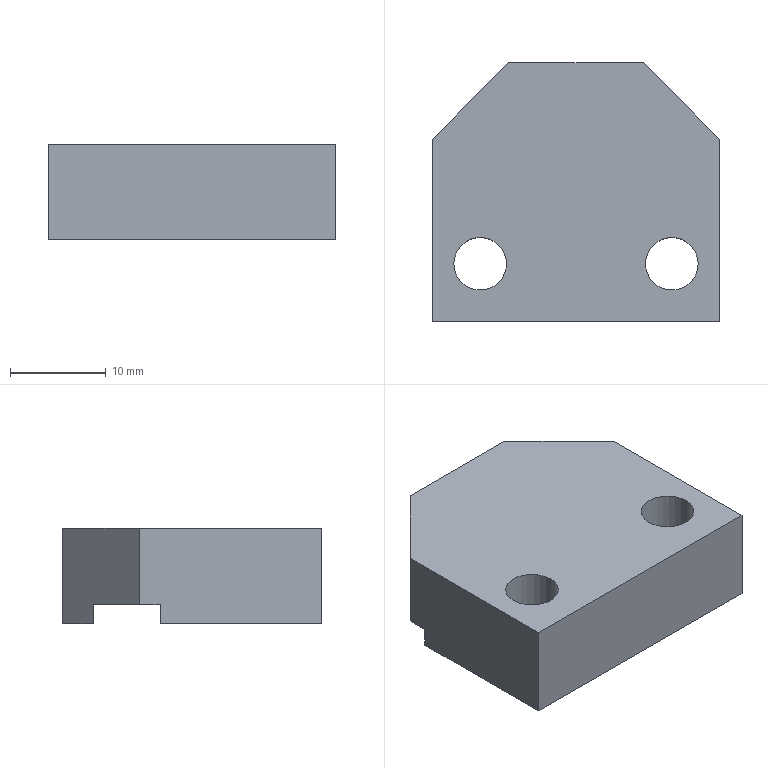Part | STEP file | detection track cover plate | 1 solid | 16 faces | box 30 x 27 x 10 mm | volume 6611 mm3 | plane 12 | cylinder 4 | commonest cylinder face diameters 5.5 x4
STEP:
#1=CARTESIAN_POINT('',(0.,0.,0.));
#2=DIRECTION('',(0.,0.,1.));
#3=DIRECTION('',(1.,0.,0.));
#4=AXIS2_PLACEMENT_3D('',#1,#2,#3);
#5=CARTESIAN_POINT('',(-12.75,-7.5,10.));
#6=VERTEX_POINT('',#5);
#7=CARTESIAN_POINT('',(-12.75,-7.5,0.));
#8=VERTEX_POINT('',#7);
#9=CARTESIAN_POINT('',(-12.75,-7.5,10.));
#10=DIRECTION('',(0.,0.,-1.));
#11=VECTOR('',#10,1.);
#12=LINE('',#9,#11);
#13=CARTESIAN_POINT('',(-10.,-7.5,10.));
#14=DIRECTION('',(0.,0.,-1.));
#15=DIRECTION('',(-1.,0.,0.));
#16=AXIS2_PLACEMENT_3D('',#13,#14,#15);
#17=CYLINDRICAL_SURFACE('',#16,2.75);
#18=CARTESIAN_POINT('',(6.283,0.));
#19=DIRECTION('',(0.,1.));
#20=VECTOR('',#19,1.);
#21=LINE('',#18,#20);
#22=(GEOMETRIC_REPRESENTATION_CONTEXT(2)PARAMETRIC_REPRESENTATION_CONTEXT()REPRESENTATION_CONTEXT('',''));
#23=DEFINITIONAL_REPRESENTATION('',(#21),#22);
#24=PCURVE('',#17,#23);
#25=CARTESIAN_POINT('',(-10.,-7.5,10.));
#26=DIRECTION('',(0.,0.,-1.));
#27=DIRECTION('',(-1.,0.,0.));
#28=AXIS2_PLACEMENT_3D('',#25,#26,#27);
#29=CYLINDRICAL_SURFACE('',#28,2.75);
#30=CARTESIAN_POINT('',(0.,0.));
#31=DIRECTION('',(0.,1.));
#32=VECTOR('',#31,1.);
#33=LINE('',#30,#32);
#34=(GEOMETRIC_REPRESENTATION_CONTEXT(2)PARAMETRIC_REPRESENTATION_CONTEXT()REPRESENTATION_CONTEXT('',''));
#35=DEFINITIONAL_REPRESENTATION('',(#33),#34);
#36=PCURVE('',#29,#35);
#37=SURFACE_CURVE('',#12,(#24,#36),.PCURVE_S1.);
#38=EDGE_CURVE('',#6,#8,#37,.T.);
#39=ORIENTED_EDGE('',*,*,#38,.T.);
#40=CARTESIAN_POINT('',(-7.25,-7.5,0.));
#41=VERTEX_POINT('',#40);
#42=CARTESIAN_POINT('',(-10.,-7.5,0.));
#43=DIRECTION('',(0.,0.,1.));
#44=DIRECTION('',(1.,0.,0.));
#45=AXIS2_PLACEMENT_3D('',#42,#43,#44);
#46=CIRCLE('',#45,2.75);
#47=CARTESIAN_POINT('',(9.425,10.));
#48=DIRECTION('',(-1.,0.));
#49=VECTOR('',#48,1.);
#50=LINE('',#47,#49);
#51=(GEOMETRIC_REPRESENTATION_CONTEXT(2)PARAMETRIC_REPRESENTATION_CONTEXT()REPRESENTATION_CONTEXT('',''));
#52=DEFINITIONAL_REPRESENTATION('',(#50),#51);
#53=PCURVE('',#17,#52);
#54=CARTESIAN_POINT('',(15.,-13.5,0.));
#55=DIRECTION('',(0.,0.,1.));
#56=DIRECTION('',(1.,0.,0.));
#57=AXIS2_PLACEMENT_3D('',#54,#55,#56);
#58=PLANE('',#57);
#59=CARTESIAN_POINT('',(-25.,6.));
#60=DIRECTION('',(1.,0.));
#61=AXIS2_PLACEMENT_2D('',#59,#60);
#62=CIRCLE('',#61,2.75);
#63=(GEOMETRIC_REPRESENTATION_CONTEXT(2)PARAMETRIC_REPRESENTATION_CONTEXT()REPRESENTATION_CONTEXT('',''));
#64=DEFINITIONAL_REPRESENTATION('',(#62),#63);
#65=PCURVE('',#58,#64);
#66=SURFACE_CURVE('',#46,(#53,#65),.PCURVE_S1.);
#67=EDGE_CURVE('',#8,#41,#66,.T.);
#68=ORIENTED_EDGE('',*,*,#67,.T.);
#69=CARTESIAN_POINT('',(-7.25,-7.5,10.));
#70=VERTEX_POINT('',#69);
#71=CARTESIAN_POINT('',(-7.25,-7.5,10.));
#72=DIRECTION('',(0.,0.,-1.));
#73=VECTOR('',#72,1.);
#74=LINE('',#71,#73);
#75=CARTESIAN_POINT('',(3.142,0.));
#76=DIRECTION('',(0.,1.));
#77=VECTOR('',#76,1.);
#78=LINE('',#75,#77);
#79=(GEOMETRIC_REPRESENTATION_CONTEXT(2)PARAMETRIC_REPRESENTATION_CONTEXT()REPRESENTATION_CONTEXT('',''));
#80=DEFINITIONAL_REPRESENTATION('',(#78),#79);
#81=PCURVE('',#17,#80);
#82=CARTESIAN_POINT('',(3.142,0.));
#83=DIRECTION('',(0.,1.));
#84=VECTOR('',#83,1.);
#85=LINE('',#82,#84);
#86=(GEOMETRIC_REPRESENTATION_CONTEXT(2)PARAMETRIC_REPRESENTATION_CONTEXT()REPRESENTATION_CONTEXT('',''));
#87=DEFINITIONAL_REPRESENTATION('',(#85),#86);
#88=PCURVE('',#29,#87);
#89=SURFACE_CURVE('',#74,(#81,#88),.PCURVE_S1.);
#90=EDGE_CURVE('',#70,#41,#89,.T.);
#91=ORIENTED_EDGE('',*,*,#90,.F.);
#92=CARTESIAN_POINT('',(-10.,-7.5,10.));
#93=DIRECTION('',(0.,0.,1.));
#94=DIRECTION('',(1.,0.,0.));
#95=AXIS2_PLACEMENT_3D('',#92,#93,#94);
#96=CIRCLE('',#95,2.75);
#97=CARTESIAN_POINT('',(9.425,0.));
#98=DIRECTION('',(-1.,0.));
#99=VECTOR('',#98,1.);
#100=LINE('',#97,#99);
#101=(GEOMETRIC_REPRESENTATION_CONTEXT(2)PARAMETRIC_REPRESENTATION_CONTEXT()REPRESENTATION_CONTEXT('',''));
#102=DEFINITIONAL_REPRESENTATION('',(#100),#101);
#103=PCURVE('',#17,#102);
#104=CARTESIAN_POINT('',(15.,-13.5,10.));
#105=DIRECTION('',(0.,0.,1.));
#106=DIRECTION('',(1.,0.,0.));
#107=AXIS2_PLACEMENT_3D('',#104,#105,#106);
#108=PLANE('',#107);
#109=CARTESIAN_POINT('',(-25.,6.));
#110=DIRECTION('',(1.,0.));
#111=AXIS2_PLACEMENT_2D('',#109,#110);
#112=CIRCLE('',#111,2.75);
#113=(GEOMETRIC_REPRESENTATION_CONTEXT(2)PARAMETRIC_REPRESENTATION_CONTEXT()REPRESENTATION_CONTEXT('',''));
#114=DEFINITIONAL_REPRESENTATION('',(#112),#113);
#115=PCURVE('',#108,#114);
#116=SURFACE_CURVE('',#96,(#103,#115),.PCURVE_S1.);
#117=EDGE_CURVE('',#6,#70,#116,.T.);
#118=ORIENTED_EDGE('',*,*,#117,.F.);
#119=EDGE_LOOP('',(#39,#68,#91,#118));
#120=FACE_BOUND('',#119,.F.);
#121=ADVANCED_FACE('',(#120),#17,.F.);
#122=CARTESIAN_POINT('',(7.25,-7.5,10.));
#123=VERTEX_POINT('',#122);
#124=CARTESIAN_POINT('',(7.25,-7.5,0.));
#125=VERTEX_POINT('',#124);
#126=CARTESIAN_POINT('',(7.25,-7.5,10.));
#127=DIRECTION('',(0.,0.,-1.));
#128=VECTOR('',#127,1.);
#129=LINE('',#126,#128);
#130=CARTESIAN_POINT('',(10.,-7.5,10.));
#131=DIRECTION('',(0.,0.,-1.));
#132=DIRECTION('',(-1.,0.,0.));
#133=AXIS2_PLACEMENT_3D('',#130,#131,#132);
#134=CYLINDRICAL_SURFACE('',#133,2.75);
#135=CARTESIAN_POINT('',(6.283,0.));
#136=DIRECTION('',(0.,1.));
#137=VECTOR('',#136,1.);
#138=LINE('',#135,#137);
#139=(GEOMETRIC_REPRESENTATION_CONTEXT(2)PARAMETRIC_REPRESENTATION_CONTEXT()REPRESENTATION_CONTEXT('',''));
#140=DEFINITIONAL_REPRESENTATION('',(#138),#139);
#141=PCURVE('',#134,#140);
#142=CARTESIAN_POINT('',(10.,-7.5,10.));
#143=DIRECTION('',(0.,0.,-1.));
#144=DIRECTION('',(-1.,0.,0.));
#145=AXIS2_PLACEMENT_3D('',#142,#143,#144);
#146=CYLINDRICAL_SURFACE('',#145,2.75);
#147=CARTESIAN_POINT('',(0.,0.));
#148=DIRECTION('',(0.,1.));
#149=VECTOR('',#148,1.);
#150=LINE('',#147,#149);
#151=(GEOMETRIC_REPRESENTATION_CONTEXT(2)PARAMETRIC_REPRESENTATION_CONTEXT()REPRESENTATION_CONTEXT('',''));
#152=DEFINITIONAL_REPRESENTATION('',(#150),#151);
#153=PCURVE('',#146,#152);
#154=SURFACE_CURVE('',#129,(#141,#153),.PCURVE_S1.);
#155=EDGE_CURVE('',#123,#125,#154,.T.);
#156=ORIENTED_EDGE('',*,*,#155,.T.);
#157=CARTESIAN_POINT('',(12.75,-7.5,0.));
#158=VERTEX_POINT('',#157);
#159=CARTESIAN_POINT('',(10.,-7.5,0.));
#160=DIRECTION('',(0.,0.,1.));
#161=DIRECTION('',(1.,0.,0.));
#162=AXIS2_PLACEMENT_3D('',#159,#160,#161);
#163=CIRCLE('',#162,2.75);
#164=CARTESIAN_POINT('',(9.425,10.));
#165=DIRECTION('',(-1.,0.));
#166=VECTOR('',#165,1.);
#167=LINE('',#164,#166);
#168=(GEOMETRIC_REPRESENTATION_CONTEXT(2)PARAMETRIC_REPRESENTATION_CONTEXT()REPRESENTATION_CONTEXT('',''));
#169=DEFINITIONAL_REPRESENTATION('',(#167),#168);
#170=PCURVE('',#134,#169);
#171=CARTESIAN_POINT('',(-5.,6.));
#172=DIRECTION('',(1.,0.));
#173=AXIS2_PLACEMENT_2D('',#171,#172);
#174=CIRCLE('',#173,2.75);
#175=(GEOMETRIC_REPRESENTATION_CONTEXT(2)PARAMETRIC_REPRESENTATION_CONTEXT()REPRESENTATION_CONTEXT('',''));
#176=DEFINITIONAL_REPRESENTATION('',(#174),#175);
#177=PCURVE('',#58,#176);
#178=SURFACE_CURVE('',#163,(#170,#177),.PCURVE_S1.);
#179=EDGE_CURVE('',#125,#158,#178,.T.);
#180=ORIENTED_EDGE('',*,*,#179,.T.);
#181=CARTESIAN_POINT('',(12.75,-7.5,10.));
#182=VERTEX_POINT('',#181);
#183=CARTESIAN_POINT('',(12.75,-7.5,10.));
#184=DIRECTION('',(0.,0.,-1.));
#185=VECTOR('',#184,1.);
#186=LINE('',#183,#185);
#187=CARTESIAN_POINT('',(3.142,0.));
#188=DIRECTION('',(0.,1.));
#189=VECTOR('',#188,1.);
#190=LINE('',#187,#189);
#191=(GEOMETRIC_REPRESENTATION_CONTEXT(2)PARAMETRIC_REPRESENTATION_CONTEXT()REPRESENTATION_CONTEXT('',''));
#192=DEFINITIONAL_REPRESENTATION('',(#190),#191);
#193=PCURVE('',#134,#192);
#194=CARTESIAN_POINT('',(3.142,0.));
#195=DIRECTION('',(0.,1.));
#196=VECTOR('',#195,1.);
#197=LINE('',#194,#196);
#198=(GEOMETRIC_REPRESENTATION_CONTEXT(2)PARAMETRIC_REPRESENTATION_CONTEXT()REPRESENTATION_CONTEXT('',''));
#199=DEFINITIONAL_REPRESENTATION('',(#197),#198);
#200=PCURVE('',#146,#199);
#201=SURFACE_CURVE('',#186,(#193,#200),.PCURVE_S1.);
#202=EDGE_CURVE('',#182,#158,#201,.T.);
#203=ORIENTED_EDGE('',*,*,#202,.F.);
#204=CARTESIAN_POINT('',(10.,-7.5,10.));
#205=DIRECTION('',(0.,0.,1.));
#206=DIRECTION('',(1.,0.,0.));
#207=AXIS2_PLACEMENT_3D('',#204,#205,#206);
#208=CIRCLE('',#207,2.75);
#209=CARTESIAN_POINT('',(9.425,0.));
#210=DIRECTION('',(-1.,0.));
#211=VECTOR('',#210,1.);
#212=LINE('',#209,#211);
#213=(GEOMETRIC_REPRESENTATION_CONTEXT(2)PARAMETRIC_REPRESENTATION_CONTEXT()REPRESENTATION_CONTEXT('',''));
#214=DEFINITIONAL_REPRESENTATION('',(#212),#213);
#215=PCURVE('',#134,#214);
#216=CARTESIAN_POINT('',(-5.,6.));
#217=DIRECTION('',(1.,0.));
#218=AXIS2_PLACEMENT_2D('',#216,#217);
#219=CIRCLE('',#218,2.75);
#220=(GEOMETRIC_REPRESENTATION_CONTEXT(2)PARAMETRIC_REPRESENTATION_CONTEXT()REPRESENTATION_CONTEXT('',''));
#221=DEFINITIONAL_REPRESENTATION('',(#219),#220);
#222=PCURVE('',#108,#221);
#223=SURFACE_CURVE('',#208,(#215,#222),.PCURVE_S1.);
#224=EDGE_CURVE('',#123,#182,#223,.T.);
#225=ORIENTED_EDGE('',*,*,#224,.F.);
#226=EDGE_LOOP('',(#156,#180,#203,#225));
#227=FACE_BOUND('',#226,.F.);
#228=ADVANCED_FACE('',(#227),#134,.F.);
#229=CARTESIAN_POINT('',(7.,13.5,0.));
#230=VERTEX_POINT('',#229);
#231=CARTESIAN_POINT('',(10.191,10.309,0.));
#232=VERTEX_POINT('',#231);
#233=CARTESIAN_POINT('',(7.,13.5,0.));
#234=DIRECTION('',(0.7071,-0.7071,0.));
#235=VECTOR('',#234,1.);
#236=LINE('',#233,#235);
#237=CARTESIAN_POINT('',(15.,-13.5,0.));
#238=DIRECTION('',(0.,0.,1.));
#239=DIRECTION('',(1.,0.,0.));
#240=AXIS2_PLACEMENT_3D('',#237,#238,#239);
#241=PLANE('',#240);
#242=CARTESIAN_POINT('',(-8.,27.));
#243=DIRECTION('',(0.7071,-0.7071));
#244=VECTOR('',#243,1.);
#245=LINE('',#242,#244);
#246=(GEOMETRIC_REPRESENTATION_CONTEXT(2)PARAMETRIC_REPRESENTATION_CONTEXT()REPRESENTATION_CONTEXT('',''));
#247=DEFINITIONAL_REPRESENTATION('',(#245),#246);
#248=PCURVE('',#241,#247);
#249=CARTESIAN_POINT('',(7.,13.5,10.));
#250=DIRECTION('',(-0.7071,-0.7071,0.));
#251=DIRECTION('',(0.7071,-0.7071,0.));
#252=AXIS2_PLACEMENT_3D('',#249,#250,#251);
#253=PLANE('',#252);
#254=CARTESIAN_POINT('',(0.,-10.));
#255=DIRECTION('',(1.,0.));
#256=VECTOR('',#255,1.);
#257=LINE('',#254,#256);
#258=(GEOMETRIC_REPRESENTATION_CONTEXT(2)PARAMETRIC_REPRESENTATION_CONTEXT()REPRESENTATION_CONTEXT('',''));
#259=DEFINITIONAL_REPRESENTATION('',(#257),#258);
#260=PCURVE('',#253,#259);
#261=SURFACE_CURVE('',#236,(#248,#260),.PCURVE_S1.);
#262=EDGE_CURVE('',#230,#232,#261,.T.);
#263=ORIENTED_EDGE('',*,*,#262,.T.);
#264=CARTESIAN_POINT('',(-10.191,10.309,0.));
#265=VERTEX_POINT('',#264);
#266=CARTESIAN_POINT('',(15.,10.309,0.));
#267=DIRECTION('',(-1.,0.,0.));
#268=VECTOR('',#267,1.);
#269=LINE('',#266,#268);
#270=CARTESIAN_POINT('',(0.,23.809));
#271=DIRECTION('',(-1.,0.));
#272=VECTOR('',#271,1.);
#273=LINE('',#270,#272);
#274=(GEOMETRIC_REPRESENTATION_CONTEXT(2)PARAMETRIC_REPRESENTATION_CONTEXT()REPRESENTATION_CONTEXT('',''));
#275=DEFINITIONAL_REPRESENTATION('',(#273),#274);
#276=PCURVE('',#241,#275);
#277=CARTESIAN_POINT('',(-15.,10.309,2.));
#278=DIRECTION('',(0.,1.,0.));
#279=DIRECTION('',(-1.,0.,0.));
#280=AXIS2_PLACEMENT_3D('',#277,#278,#279);
#281=PLANE('',#280);
#282=CARTESIAN_POINT('',(-30.,-2.));
#283=DIRECTION('',(1.,0.));
#284=VECTOR('',#283,1.);
#285=LINE('',#282,#284);
#286=(GEOMETRIC_REPRESENTATION_CONTEXT(2)PARAMETRIC_REPRESENTATION_CONTEXT()REPRESENTATION_CONTEXT('',''));
#287=DEFINITIONAL_REPRESENTATION('',(#285),#286);
#288=PCURVE('',#281,#287);
#289=SURFACE_CURVE('',#269,(#276,#288),.PCURVE_S1.);
#290=EDGE_CURVE('',#232,#265,#289,.T.);
#291=ORIENTED_EDGE('',*,*,#290,.T.);
#292=CARTESIAN_POINT('',(-7.,13.5,0.));
#293=VERTEX_POINT('',#292);
#294=CARTESIAN_POINT('',(-15.,5.5,0.));
#295=DIRECTION('',(0.7071,0.7071,0.));
#296=VECTOR('',#295,1.);
#297=LINE('',#294,#296);
#298=CARTESIAN_POINT('',(-30.,19.));
#299=DIRECTION('',(0.7071,0.7071));
#300=VECTOR('',#299,1.);
#301=LINE('',#298,#300);
#302=(GEOMETRIC_REPRESENTATION_CONTEXT(2)PARAMETRIC_REPRESENTATION_CONTEXT()REPRESENTATION_CONTEXT('',''));
#303=DEFINITIONAL_REPRESENTATION('',(#301),#302);
#304=PCURVE('',#241,#303);
#305=CARTESIAN_POINT('',(-15.,5.5,10.));
#306=DIRECTION('',(0.7071,-0.7071,0.));
#307=DIRECTION('',(0.7071,0.7071,0.));
#308=AXIS2_PLACEMENT_3D('',#305,#306,#307);
#309=PLANE('',#308);
#310=CARTESIAN_POINT('',(0.,-10.));
#311=DIRECTION('',(1.,0.));
#312=VECTOR('',#311,1.);
#313=LINE('',#310,#312);
#314=(GEOMETRIC_REPRESENTATION_CONTEXT(2)PARAMETRIC_REPRESENTATION_CONTEXT()REPRESENTATION_CONTEXT('',''));
#315=DEFINITIONAL_REPRESENTATION('',(#313),#314);
#316=PCURVE('',#309,#315);
#317=SURFACE_CURVE('',#297,(#304,#316),.PCURVE_S1.);
#318=EDGE_CURVE('',#265,#293,#317,.T.);
#319=ORIENTED_EDGE('',*,*,#318,.T.);
#320=CARTESIAN_POINT('',(-15.,13.5,0.));
#321=DIRECTION('',(-1.,0.,0.));
#322=VECTOR('',#321,1.);
#323=LINE('',#320,#322);
#324=CARTESIAN_POINT('',(-30.,27.));
#325=DIRECTION('',(-1.,0.));
#326=VECTOR('',#325,1.);
#327=LINE('',#324,#326);
#328=(GEOMETRIC_REPRESENTATION_CONTEXT(2)PARAMETRIC_REPRESENTATION_CONTEXT()REPRESENTATION_CONTEXT('',''));
#329=DEFINITIONAL_REPRESENTATION('',(#327),#328);
#330=PCURVE('',#241,#329);
#331=CARTESIAN_POINT('',(-15.,13.5,10.));
#332=DIRECTION('',(0.,-1.,0.));
#333=DIRECTION('',(0.,0.,-1.));
#334=AXIS2_PLACEMENT_3D('',#331,#332,#333);
#335=PLANE('',#334);
#336=CARTESIAN_POINT('',(10.,0.));
#337=DIRECTION('',(0.,-1.));
#338=VECTOR('',#337,1.);
#339=LINE('',#336,#338);
#340=(GEOMETRIC_REPRESENTATION_CONTEXT(2)PARAMETRIC_REPRESENTATION_CONTEXT()REPRESENTATION_CONTEXT('',''));
#341=DEFINITIONAL_REPRESENTATION('',(#339),#340);
#342=PCURVE('',#335,#341);
#343=SURFACE_CURVE('',#323,(#330,#342),.PCURVE_S1.);
#344=EDGE_CURVE('',#230,#293,#343,.T.);
#345=ORIENTED_EDGE('',*,*,#344,.F.);
#346=EDGE_LOOP('',(#263,#291,#319,#345));
#347=FACE_BOUND('',#346,.T.);
#348=ADVANCED_FACE('',(#347),#241,.F.);
#349=ORIENTED_EDGE('',*,*,#224,.F.);
#350=CARTESIAN_POINT('',(10.,-7.5,10.));
#351=DIRECTION('',(0.,0.,1.));
#352=DIRECTION('',(1.,0.,0.));
#353=AXIS2_PLACEMENT_3D('',#350,#351,#352);
#354=CIRCLE('',#353,2.75);
#355=CARTESIAN_POINT('',(-5.,6.));
#356=DIRECTION('',(1.,0.));
#357=AXIS2_PLACEMENT_2D('',#355,#356);
#358=CIRCLE('',#357,2.75);
#359=(GEOMETRIC_REPRESENTATION_CONTEXT(2)PARAMETRIC_REPRESENTATION_CONTEXT()REPRESENTATION_CONTEXT('',''));
#360=DEFINITIONAL_REPRESENTATION('',(#358),#359);
#361=PCURVE('',#108,#360);
#362=CARTESIAN_POINT('',(3.142,0.));
#363=DIRECTION('',(-1.,0.));
#364=VECTOR('',#363,1.);
#365=LINE('',#362,#364);
#366=(GEOMETRIC_REPRESENTATION_CONTEXT(2)PARAMETRIC_REPRESENTATION_CONTEXT()REPRESENTATION_CONTEXT('',''));
#367=DEFINITIONAL_REPRESENTATION('',(#365),#366);
#368=PCURVE('',#146,#367);
#369=SURFACE_CURVE('',#354,(#361,#368),.PCURVE_S1.);
#370=EDGE_CURVE('',#182,#123,#369,.T.);
#371=ORIENTED_EDGE('',*,*,#370,.F.);
#372=EDGE_LOOP('',(#349,#371));
#373=FACE_BOUND('',#372,.T.);
#374=CARTESIAN_POINT('',(7.,13.5,10.));
#375=VERTEX_POINT('',#374);
#376=CARTESIAN_POINT('',(-7.,13.5,10.));
#377=VERTEX_POINT('',#376);
#378=CARTESIAN_POINT('',(-15.,13.5,10.));
#379=DIRECTION('',(-1.,0.,0.));
#380=VECTOR('',#379,1.);
#381=LINE('',#378,#380);
#382=CARTESIAN_POINT('',(-30.,27.));
#383=DIRECTION('',(-1.,0.));
#384=VECTOR('',#383,1.);
#385=LINE('',#382,#384);
#386=(GEOMETRIC_REPRESENTATION_CONTEXT(2)PARAMETRIC_REPRESENTATION_CONTEXT()REPRESENTATION_CONTEXT('',''));
#387=DEFINITIONAL_REPRESENTATION('',(#385),#386);
#388=PCURVE('',#108,#387);
#389=CARTESIAN_POINT('',(0.,0.));
#390=DIRECTION('',(0.,-1.));
#391=VECTOR('',#390,1.);
#392=LINE('',#389,#391);
#393=(GEOMETRIC_REPRESENTATION_CONTEXT(2)PARAMETRIC_REPRESENTATION_CONTEXT()REPRESENTATION_CONTEXT('',''));
#394=DEFINITIONAL_REPRESENTATION('',(#392),#393);
#395=PCURVE('',#335,#394);
#396=SURFACE_CURVE('',#381,(#388,#395),.PCURVE_S1.);
#397=EDGE_CURVE('',#375,#377,#396,.T.);
#398=ORIENTED_EDGE('',*,*,#397,.T.);
#399=CARTESIAN_POINT('',(-15.,5.5,10.));
#400=VERTEX_POINT('',#399);
#401=CARTESIAN_POINT('',(-9.5,11.,10.));
#402=DIRECTION('',(-0.7071,-0.7071,0.));
#403=VECTOR('',#402,1.);
#404=LINE('',#401,#403);
#405=CARTESIAN_POINT('',(-24.5,24.5));
#406=DIRECTION('',(-0.7071,-0.7071));
#407=VECTOR('',#406,1.);
#408=LINE('',#405,#407);
#409=(GEOMETRIC_REPRESENTATION_CONTEXT(2)PARAMETRIC_REPRESENTATION_CONTEXT()REPRESENTATION_CONTEXT('',''));
#410=DEFINITIONAL_REPRESENTATION('',(#408),#409);
#411=PCURVE('',#108,#410);
#412=CARTESIAN_POINT('',(7.778,0.));
#413=DIRECTION('',(-1.,0.));
#414=VECTOR('',#413,1.);
#415=LINE('',#412,#414);
#416=(GEOMETRIC_REPRESENTATION_CONTEXT(2)PARAMETRIC_REPRESENTATION_CONTEXT()REPRESENTATION_CONTEXT('',''));
#417=DEFINITIONAL_REPRESENTATION('',(#415),#416);
#418=PCURVE('',#309,#417);
#419=SURFACE_CURVE('',#404,(#411,#418),.PCURVE_S1.);
#420=EDGE_CURVE('',#377,#400,#419,.T.);
#421=ORIENTED_EDGE('',*,*,#420,.T.);
#422=CARTESIAN_POINT('',(-15.,-13.5,10.));
#423=VERTEX_POINT('',#422);
#424=CARTESIAN_POINT('',(-15.,13.5,10.));
#425=DIRECTION('',(0.,-1.,0.));
#426=VECTOR('',#425,1.);
#427=LINE('',#424,#426);
#428=CARTESIAN_POINT('',(-30.,27.));
#429=DIRECTION('',(0.,-1.));
#430=VECTOR('',#429,1.);
#431=LINE('',#428,#430);
#432=(GEOMETRIC_REPRESENTATION_CONTEXT(2)PARAMETRIC_REPRESENTATION_CONTEXT()REPRESENTATION_CONTEXT('',''));
#433=DEFINITIONAL_REPRESENTATION('',(#431),#432);
#434=PCURVE('',#108,#433);
#435=CARTESIAN_POINT('',(-15.,13.5,10.));
#436=DIRECTION('',(1.,0.,0.));
#437=DIRECTION('',(0.,1.,0.));
#438=AXIS2_PLACEMENT_3D('',#435,#436,#437);
#439=PLANE('',#438);
#440=CARTESIAN_POINT('',(0.,0.));
#441=DIRECTION('',(-1.,0.));
#442=VECTOR('',#441,1.);
#443=LINE('',#440,#442);
#444=(GEOMETRIC_REPRESENTATION_CONTEXT(2)PARAMETRIC_REPRESENTATION_CONTEXT()REPRESENTATION_CONTEXT('',''));
#445=DEFINITIONAL_REPRESENTATION('',(#443),#444);
#446=PCURVE('',#439,#445);
#447=SURFACE_CURVE('',#427,(#434,#446),.PCURVE_S1.);
#448=EDGE_CURVE('',#400,#423,#447,.T.);
#449=ORIENTED_EDGE('',*,*,#448,.T.);
#450=CARTESIAN_POINT('',(15.,-13.5,10.));
#451=VERTEX_POINT('',#450);
#452=CARTESIAN_POINT('',(-15.,-13.5,10.));
#453=DIRECTION('',(1.,0.,0.));
#454=VECTOR('',#453,1.);
#455=LINE('',#452,#454);
#456=CARTESIAN_POINT('',(-30.,0.));
#457=DIRECTION('',(1.,0.));
#458=VECTOR('',#457,1.);
#459=LINE('',#456,#458);
#460=(GEOMETRIC_REPRESENTATION_CONTEXT(2)PARAMETRIC_REPRESENTATION_CONTEXT()REPRESENTATION_CONTEXT('',''));
#461=DEFINITIONAL_REPRESENTATION('',(#459),#460);
#462=PCURVE('',#108,#461);
#463=CARTESIAN_POINT('',(-15.,-13.5,10.));
#464=DIRECTION('',(0.,1.,0.));
#465=DIRECTION('',(0.,0.,1.));
#466=AXIS2_PLACEMENT_3D('',#463,#464,#465);
#467=PLANE('',#466);
#468=CARTESIAN_POINT('',(0.,0.));
#469=DIRECTION('',(0.,1.));
#470=VECTOR('',#469,1.);
#471=LINE('',#468,#470);
#472=(GEOMETRIC_REPRESENTATION_CONTEXT(2)PARAMETRIC_REPRESENTATION_CONTEXT()REPRESENTATION_CONTEXT('',''));
#473=DEFINITIONAL_REPRESENTATION('',(#471),#472);
#474=PCURVE('',#467,#473);
#475=SURFACE_CURVE('',#455,(#462,#474),.PCURVE_S1.);
#476=EDGE_CURVE('',#423,#451,#475,.T.);
#477=ORIENTED_EDGE('',*,*,#476,.T.);
#478=CARTESIAN_POINT('',(15.,5.5,10.));
#479=VERTEX_POINT('',#478);
#480=CARTESIAN_POINT('',(15.,13.5,10.));
#481=DIRECTION('',(0.,1.,0.));
#482=VECTOR('',#481,1.);
#483=LINE('',#480,#482);
#484=CARTESIAN_POINT('',(0.,27.));
#485=DIRECTION('',(0.,1.));
#486=VECTOR('',#485,1.);
#487=LINE('',#484,#486);
#488=(GEOMETRIC_REPRESENTATION_CONTEXT(2)PARAMETRIC_REPRESENTATION_CONTEXT()REPRESENTATION_CONTEXT('',''));
#489=DEFINITIONAL_REPRESENTATION('',(#487),#488);
#490=PCURVE('',#108,#489);
#491=CARTESIAN_POINT('',(15.,13.5,10.));
#492=DIRECTION('',(-1.,0.,0.));
#493=DIRECTION('',(0.,-1.,0.));
#494=AXIS2_PLACEMENT_3D('',#491,#492,#493);
#495=PLANE('',#494);
#496=CARTESIAN_POINT('',(0.,0.));
#497=DIRECTION('',(-1.,0.));
#498=VECTOR('',#497,1.);
#499=LINE('',#496,#498);
#500=(GEOMETRIC_REPRESENTATION_CONTEXT(2)PARAMETRIC_REPRESENTATION_CONTEXT()REPRESENTATION_CONTEXT('',''));
#501=DEFINITIONAL_REPRESENTATION('',(#499),#500);
#502=PCURVE('',#495,#501);
#503=SURFACE_CURVE('',#483,(#490,#502),.PCURVE_S1.);
#504=EDGE_CURVE('',#451,#479,#503,.T.);
#505=ORIENTED_EDGE('',*,*,#504,.T.);
#506=CARTESIAN_POINT('',(24.5,-4.,10.));
#507=DIRECTION('',(-0.7071,0.7071,0.));
#508=VECTOR('',#507,1.);
#509=LINE('',#506,#508);
#510=CARTESIAN_POINT('',(9.5,9.5));
#511=DIRECTION('',(-0.7071,0.7071));
#512=VECTOR('',#511,1.);
#513=LINE('',#510,#512);
#514=(GEOMETRIC_REPRESENTATION_CONTEXT(2)PARAMETRIC_REPRESENTATION_CONTEXT()REPRESENTATION_CONTEXT('',''));
#515=DEFINITIONAL_REPRESENTATION('',(#513),#514);
#516=PCURVE('',#108,#515);
#517=CARTESIAN_POINT('',(24.749,0.));
#518=DIRECTION('',(-1.,0.));
#519=VECTOR('',#518,1.);
#520=LINE('',#517,#519);
#521=(GEOMETRIC_REPRESENTATION_CONTEXT(2)PARAMETRIC_REPRESENTATION_CONTEXT()REPRESENTATION_CONTEXT('',''));
#522=DEFINITIONAL_REPRESENTATION('',(#520),#521);
#523=PCURVE('',#253,#522);
#524=SURFACE_CURVE('',#509,(#516,#523),.PCURVE_S1.);
#525=EDGE_CURVE('',#479,#375,#524,.T.);
#526=ORIENTED_EDGE('',*,*,#525,.T.);
#527=EDGE_LOOP('',(#398,#421,#449,#477,#505,#526));
#528=FACE_BOUND('',#527,.T.);
#529=ORIENTED_EDGE('',*,*,#117,.F.);
#530=CARTESIAN_POINT('',(-10.,-7.5,10.));
#531=DIRECTION('',(0.,0.,1.));
#532=DIRECTION('',(1.,0.,0.));
#533=AXIS2_PLACEMENT_3D('',#530,#531,#532);
#534=CIRCLE('',#533,2.75);
#535=CARTESIAN_POINT('',(-25.,6.));
#536=DIRECTION('',(1.,0.));
#537=AXIS2_PLACEMENT_2D('',#535,#536);
#538=CIRCLE('',#537,2.75);
#539=(GEOMETRIC_REPRESENTATION_CONTEXT(2)PARAMETRIC_REPRESENTATION_CONTEXT()REPRESENTATION_CONTEXT('',''));
#540=DEFINITIONAL_REPRESENTATION('',(#538),#539);
#541=PCURVE('',#108,#540);
#542=CARTESIAN_POINT('',(3.142,0.));
#543=DIRECTION('',(-1.,0.));
#544=VECTOR('',#543,1.);
#545=LINE('',#542,#544);
#546=(GEOMETRIC_REPRESENTATION_CONTEXT(2)PARAMETRIC_REPRESENTATION_CONTEXT()REPRESENTATION_CONTEXT('',''));
#547=DEFINITIONAL_REPRESENTATION('',(#545),#546);
#548=PCURVE('',#29,#547);
#549=SURFACE_CURVE('',#534,(#541,#548),.PCURVE_S1.);
#550=EDGE_CURVE('',#70,#6,#549,.T.);
#551=ORIENTED_EDGE('',*,*,#550,.F.);
#552=EDGE_LOOP('',(#529,#551));
#553=FACE_BOUND('',#552,.T.);
#554=ADVANCED_FACE('',(#373,#528,#553),#108,.T.);
#555=ORIENTED_EDGE('',*,*,#179,.T.);
#556=CARTESIAN_POINT('',(10.,-7.5,0.));
#557=DIRECTION('',(0.,0.,1.));
#558=DIRECTION('',(1.,0.,0.));
#559=AXIS2_PLACEMENT_3D('',#556,#557,#558);
#560=CIRCLE('',#559,2.75);
#561=CARTESIAN_POINT('',(-5.,6.));
#562=DIRECTION('',(1.,0.));
#563=AXIS2_PLACEMENT_2D('',#561,#562);
#564=CIRCLE('',#563,2.75);
#565=(GEOMETRIC_REPRESENTATION_CONTEXT(2)PARAMETRIC_REPRESENTATION_CONTEXT()REPRESENTATION_CONTEXT('',''));
#566=DEFINITIONAL_REPRESENTATION('',(#564),#565);
#567=PCURVE('',#58,#566);
#568=CARTESIAN_POINT('',(3.142,10.));
#569=DIRECTION('',(-1.,0.));
#570=VECTOR('',#569,1.);
#571=LINE('',#568,#570);
#572=(GEOMETRIC_REPRESENTATION_CONTEXT(2)PARAMETRIC_REPRESENTATION_CONTEXT()REPRESENTATION_CONTEXT('',''));
#573=DEFINITIONAL_REPRESENTATION('',(#571),#572);
#574=PCURVE('',#146,#573);
#575=SURFACE_CURVE('',#560,(#567,#574),.PCURVE_S1.);
#576=EDGE_CURVE('',#158,#125,#575,.T.);
#577=ORIENTED_EDGE('',*,*,#576,.T.);
#578=EDGE_LOOP('',(#555,#577));
#579=FACE_BOUND('',#578,.T.);
#580=CARTESIAN_POINT('',(-15.,3.309,0.));
#581=VERTEX_POINT('',#580);
#582=CARTESIAN_POINT('',(-15.,-13.5,0.));
#583=VERTEX_POINT('',#582);
#584=CARTESIAN_POINT('',(-15.,13.5,0.));
#585=DIRECTION('',(0.,-1.,0.));
#586=VECTOR('',#585,1.);
#587=LINE('',#584,#586);
#588=CARTESIAN_POINT('',(-30.,27.));
#589=DIRECTION('',(0.,-1.));
#590=VECTOR('',#589,1.);
#591=LINE('',#588,#590);
#592=(GEOMETRIC_REPRESENTATION_CONTEXT(2)PARAMETRIC_REPRESENTATION_CONTEXT()REPRESENTATION_CONTEXT('',''));
#593=DEFINITIONAL_REPRESENTATION('',(#591),#592);
#594=PCURVE('',#58,#593);
#595=CARTESIAN_POINT('',(0.,-10.));
#596=DIRECTION('',(-1.,0.));
#597=VECTOR('',#596,1.);
#598=LINE('',#595,#597);
#599=(GEOMETRIC_REPRESENTATION_CONTEXT(2)PARAMETRIC_REPRESENTATION_CONTEXT()REPRESENTATION_CONTEXT('',''));
#600=DEFINITIONAL_REPRESENTATION('',(#598),#599);
#601=PCURVE('',#439,#600);
#602=SURFACE_CURVE('',#587,(#594,#601),.PCURVE_S1.);
#603=EDGE_CURVE('',#581,#583,#602,.T.);
#604=ORIENTED_EDGE('',*,*,#603,.F.);
#605=CARTESIAN_POINT('',(15.,3.309,0.));
#606=VERTEX_POINT('',#605);
#607=CARTESIAN_POINT('',(15.,3.309,0.));
#608=DIRECTION('',(1.,0.,0.));
#609=VECTOR('',#608,1.);
#610=LINE('',#607,#609);
#611=CARTESIAN_POINT('',(0.,16.809));
#612=DIRECTION('',(1.,0.));
#613=VECTOR('',#612,1.);
#614=LINE('',#611,#613);
#615=(GEOMETRIC_REPRESENTATION_CONTEXT(2)PARAMETRIC_REPRESENTATION_CONTEXT()REPRESENTATION_CONTEXT('',''));
#616=DEFINITIONAL_REPRESENTATION('',(#614),#615);
#617=PCURVE('',#58,#616);
#618=CARTESIAN_POINT('',(-15.,3.309,2.));
#619=DIRECTION('',(0.,-1.,0.));
#620=DIRECTION('',(1.,0.,0.));
#621=AXIS2_PLACEMENT_3D('',#618,#619,#620);
#622=PLANE('',#621);
#623=CARTESIAN_POINT('',(30.,-2.));
#624=DIRECTION('',(1.,0.));
#625=VECTOR('',#624,1.);
#626=LINE('',#623,#625);
#627=(GEOMETRIC_REPRESENTATION_CONTEXT(2)PARAMETRIC_REPRESENTATION_CONTEXT()REPRESENTATION_CONTEXT('',''));
#628=DEFINITIONAL_REPRESENTATION('',(#626),#627);
#629=PCURVE('',#622,#628);
#630=SURFACE_CURVE('',#610,(#617,#629),.PCURVE_S1.);
#631=EDGE_CURVE('',#581,#606,#630,.T.);
#632=ORIENTED_EDGE('',*,*,#631,.T.);
#633=CARTESIAN_POINT('',(15.,-13.5,0.));
#634=VERTEX_POINT('',#633);
#635=CARTESIAN_POINT('',(15.,13.5,0.));
#636=DIRECTION('',(0.,1.,0.));
#637=VECTOR('',#636,1.);
#638=LINE('',#635,#637);
#639=CARTESIAN_POINT('',(0.,27.));
#640=DIRECTION('',(0.,1.));
#641=VECTOR('',#640,1.);
#642=LINE('',#639,#641);
#643=(GEOMETRIC_REPRESENTATION_CONTEXT(2)PARAMETRIC_REPRESENTATION_CONTEXT()REPRESENTATION_CONTEXT('',''));
#644=DEFINITIONAL_REPRESENTATION('',(#642),#643);
#645=PCURVE('',#58,#644);
#646=CARTESIAN_POINT('',(0.,-10.));
#647=DIRECTION('',(-1.,0.));
#648=VECTOR('',#647,1.);
#649=LINE('',#646,#648);
#650=(GEOMETRIC_REPRESENTATION_CONTEXT(2)PARAMETRIC_REPRESENTATION_CONTEXT()REPRESENTATION_CONTEXT('',''));
#651=DEFINITIONAL_REPRESENTATION('',(#649),#650);
#652=PCURVE('',#495,#651);
#653=SURFACE_CURVE('',#638,(#645,#652),.PCURVE_S1.);
#654=EDGE_CURVE('',#634,#606,#653,.T.);
#655=ORIENTED_EDGE('',*,*,#654,.F.);
#656=CARTESIAN_POINT('',(-15.,-13.5,0.));
#657=DIRECTION('',(1.,0.,0.));
#658=VECTOR('',#657,1.);
#659=LINE('',#656,#658);
#660=CARTESIAN_POINT('',(-30.,0.));
#661=DIRECTION('',(1.,0.));
#662=VECTOR('',#661,1.);
#663=LINE('',#660,#662);
#664=(GEOMETRIC_REPRESENTATION_CONTEXT(2)PARAMETRIC_REPRESENTATION_CONTEXT()REPRESENTATION_CONTEXT('',''));
#665=DEFINITIONAL_REPRESENTATION('',(#663),#664);
#666=PCURVE('',#58,#665);
#667=CARTESIAN_POINT('',(-10.,0.));
#668=DIRECTION('',(0.,1.));
#669=VECTOR('',#668,1.);
#670=LINE('',#667,#669);
#671=(GEOMETRIC_REPRESENTATION_CONTEXT(2)PARAMETRIC_REPRESENTATION_CONTEXT()REPRESENTATION_CONTEXT('',''));
#672=DEFINITIONAL_REPRESENTATION('',(#670),#671);
#673=PCURVE('',#467,#672);
#674=SURFACE_CURVE('',#659,(#666,#673),.PCURVE_S1.);
#675=EDGE_CURVE('',#583,#634,#674,.T.);
#676=ORIENTED_EDGE('',*,*,#675,.F.);
#677=EDGE_LOOP('',(#604,#632,#655,#676));
#678=FACE_BOUND('',#677,.T.);
#679=ORIENTED_EDGE('',*,*,#67,.T.);
#680=CARTESIAN_POINT('',(-10.,-7.5,0.));
#681=DIRECTION('',(0.,0.,1.));
#682=DIRECTION('',(1.,0.,0.));
#683=AXIS2_PLACEMENT_3D('',#680,#681,#682);
#684=CIRCLE('',#683,2.75);
#685=CARTESIAN_POINT('',(-25.,6.));
#686=DIRECTION('',(1.,0.));
#687=AXIS2_PLACEMENT_2D('',#685,#686);
#688=CIRCLE('',#687,2.75);
#689=(GEOMETRIC_REPRESENTATION_CONTEXT(2)PARAMETRIC_REPRESENTATION_CONTEXT()REPRESENTATION_CONTEXT('',''));
#690=DEFINITIONAL_REPRESENTATION('',(#688),#689);
#691=PCURVE('',#58,#690);
#692=CARTESIAN_POINT('',(3.142,10.));
#693=DIRECTION('',(-1.,0.));
#694=VECTOR('',#693,1.);
#695=LINE('',#692,#694);
#696=(GEOMETRIC_REPRESENTATION_CONTEXT(2)PARAMETRIC_REPRESENTATION_CONTEXT()REPRESENTATION_CONTEXT('',''));
#697=DEFINITIONAL_REPRESENTATION('',(#695),#696);
#698=PCURVE('',#29,#697);
#699=SURFACE_CURVE('',#684,(#691,#698),.PCURVE_S1.);
#700=EDGE_CURVE('',#41,#8,#699,.T.);
#701=ORIENTED_EDGE('',*,*,#700,.T.);
#702=EDGE_LOOP('',(#679,#701));
#703=FACE_BOUND('',#702,.T.);
#704=ADVANCED_FACE('',(#579,#678,#703),#58,.F.);
#705=CARTESIAN_POINT('',(15.,3.309,2.));
#706=VERTEX_POINT('',#705);
#707=CARTESIAN_POINT('',(15.,3.309,2.));
#708=DIRECTION('',(0.,0.,-1.));
#709=VECTOR('',#708,1.);
#710=LINE('',#707,#709);
#711=CARTESIAN_POINT('',(10.191,-8.));
#712=DIRECTION('',(0.,-1.));
#713=VECTOR('',#712,1.);
#714=LINE('',#711,#713);
#715=(GEOMETRIC_REPRESENTATION_CONTEXT(2)PARAMETRIC_REPRESENTATION_CONTEXT()REPRESENTATION_CONTEXT('',''));
#716=DEFINITIONAL_REPRESENTATION('',(#714),#715);
#717=PCURVE('',#495,#716);
#718=CARTESIAN_POINT('',(30.,0.));
#719=DIRECTION('',(0.,-1.));
#720=VECTOR('',#719,1.);
#721=LINE('',#718,#720);
#722=(GEOMETRIC_REPRESENTATION_CONTEXT(2)PARAMETRIC_REPRESENTATION_CONTEXT()REPRESENTATION_CONTEXT('',''));
#723=DEFINITIONAL_REPRESENTATION('',(#721),#722);
#724=PCURVE('',#622,#723);
#725=SURFACE_CURVE('',#710,(#717,#724),.PCURVE_S1.);
#726=EDGE_CURVE('',#706,#606,#725,.T.);
#727=ORIENTED_EDGE('',*,*,#726,.F.);
#728=CARTESIAN_POINT('',(15.,5.5,2.));
#729=VERTEX_POINT('',#728);
#730=CARTESIAN_POINT('',(15.,10.309,2.));
#731=DIRECTION('',(0.,-1.,0.));
#732=VECTOR('',#731,1.);
#733=LINE('',#730,#732);
#734=CARTESIAN_POINT('',(3.191,-8.));
#735=DIRECTION('',(1.,0.));
#736=VECTOR('',#735,1.);
#737=LINE('',#734,#736);
#738=(GEOMETRIC_REPRESENTATION_CONTEXT(2)PARAMETRIC_REPRESENTATION_CONTEXT()REPRESENTATION_CONTEXT('',''));
#739=DEFINITIONAL_REPRESENTATION('',(#737),#738);
#740=PCURVE('',#495,#739);
#741=CARTESIAN_POINT('',(-15.,10.309,2.));
#742=DIRECTION('',(0.,0.,1.));
#743=DIRECTION('',(1.,0.,0.));
#744=AXIS2_PLACEMENT_3D('',#741,#742,#743);
#745=PLANE('',#744);
#746=CARTESIAN_POINT('',(30.,0.));
#747=DIRECTION('',(0.,-1.));
#748=VECTOR('',#747,1.);
#749=LINE('',#746,#748);
#750=(GEOMETRIC_REPRESENTATION_CONTEXT(2)PARAMETRIC_REPRESENTATION_CONTEXT()REPRESENTATION_CONTEXT('',''));
#751=DEFINITIONAL_REPRESENTATION('',(#749),#750);
#752=PCURVE('',#745,#751);
#753=SURFACE_CURVE('',#733,(#740,#752),.PCURVE_S1.);
#754=EDGE_CURVE('',#729,#706,#753,.T.);
#755=ORIENTED_EDGE('',*,*,#754,.F.);
#756=CARTESIAN_POINT('',(15.,5.5,10.));
#757=DIRECTION('',(0.,0.,1.));
#758=VECTOR('',#757,1.);
#759=LINE('',#756,#758);
#760=CARTESIAN_POINT('',(8.,0.));
#761=DIRECTION('',(0.,1.));
#762=VECTOR('',#761,1.);
#763=LINE('',#760,#762);
#764=(GEOMETRIC_REPRESENTATION_CONTEXT(2)PARAMETRIC_REPRESENTATION_CONTEXT()REPRESENTATION_CONTEXT('',''));
#765=DEFINITIONAL_REPRESENTATION('',(#763),#764);
#766=PCURVE('',#495,#765);
#767=CARTESIAN_POINT('',(11.314,0.));
#768=DIRECTION('',(0.,1.));
#769=VECTOR('',#768,1.);
#770=LINE('',#767,#769);
#771=(GEOMETRIC_REPRESENTATION_CONTEXT(2)PARAMETRIC_REPRESENTATION_CONTEXT()REPRESENTATION_CONTEXT('',''));
#772=DEFINITIONAL_REPRESENTATION('',(#770),#771);
#773=PCURVE('',#253,#772);
#774=SURFACE_CURVE('',#759,(#766,#773),.PCURVE_S1.);
#775=EDGE_CURVE('',#729,#479,#774,.T.);
#776=ORIENTED_EDGE('',*,*,#775,.T.);
#777=ORIENTED_EDGE('',*,*,#504,.F.);
#778=CARTESIAN_POINT('',(15.,-13.5,10.));
#779=DIRECTION('',(0.,0.,-1.));
#780=VECTOR('',#779,1.);
#781=LINE('',#778,#780);
#782=CARTESIAN_POINT('',(27.,0.));
#783=DIRECTION('',(0.,-1.));
#784=VECTOR('',#783,1.);
#785=LINE('',#782,#784);
#786=(GEOMETRIC_REPRESENTATION_CONTEXT(2)PARAMETRIC_REPRESENTATION_CONTEXT()REPRESENTATION_CONTEXT('',''));
#787=DEFINITIONAL_REPRESENTATION('',(#785),#786);
#788=PCURVE('',#495,#787);
#789=CARTESIAN_POINT('',(0.,30.));
#790=DIRECTION('',(-1.,0.));
#791=VECTOR('',#790,1.);
#792=LINE('',#789,#791);
#793=(GEOMETRIC_REPRESENTATION_CONTEXT(2)PARAMETRIC_REPRESENTATION_CONTEXT()REPRESENTATION_CONTEXT('',''));
#794=DEFINITIONAL_REPRESENTATION('',(#792),#793);
#795=PCURVE('',#467,#794);
#796=SURFACE_CURVE('',#781,(#788,#795),.PCURVE_S1.);
#797=EDGE_CURVE('',#451,#634,#796,.T.);
#798=ORIENTED_EDGE('',*,*,#797,.T.);
#799=ORIENTED_EDGE('',*,*,#654,.T.);
#800=EDGE_LOOP('',(#727,#755,#776,#777,#798,#799));
#801=FACE_BOUND('',#800,.T.);
#802=ADVANCED_FACE('',(#801),#495,.F.);
#803=ORIENTED_EDGE('',*,*,#344,.T.);
#804=CARTESIAN_POINT('',(-7.,13.5,10.));
#805=DIRECTION('',(0.,0.,1.));
#806=VECTOR('',#805,1.);
#807=LINE('',#804,#806);
#808=CARTESIAN_POINT('',(0.,8.));
#809=DIRECTION('',(-1.,0.));
#810=VECTOR('',#809,1.);
#811=LINE('',#808,#810);
#812=(GEOMETRIC_REPRESENTATION_CONTEXT(2)PARAMETRIC_REPRESENTATION_CONTEXT()REPRESENTATION_CONTEXT('',''));
#813=DEFINITIONAL_REPRESENTATION('',(#811),#812);
#814=PCURVE('',#335,#813);
#815=CARTESIAN_POINT('',(11.314,0.));
#816=DIRECTION('',(0.,1.));
#817=VECTOR('',#816,1.);
#818=LINE('',#815,#817);
#819=(GEOMETRIC_REPRESENTATION_CONTEXT(2)PARAMETRIC_REPRESENTATION_CONTEXT()REPRESENTATION_CONTEXT('',''));
#820=DEFINITIONAL_REPRESENTATION('',(#818),#819);
#821=PCURVE('',#309,#820);
#822=SURFACE_CURVE('',#807,(#814,#821),.PCURVE_S1.);
#823=EDGE_CURVE('',#293,#377,#822,.T.);
#824=ORIENTED_EDGE('',*,*,#823,.T.);
#825=ORIENTED_EDGE('',*,*,#397,.F.);
#826=CARTESIAN_POINT('',(7.,13.5,10.));
#827=DIRECTION('',(0.,0.,-1.));
#828=VECTOR('',#827,1.);
#829=LINE('',#826,#828);
#830=CARTESIAN_POINT('',(0.,22.));
#831=DIRECTION('',(1.,0.));
#832=VECTOR('',#831,1.);
#833=LINE('',#830,#832);
#834=(GEOMETRIC_REPRESENTATION_CONTEXT(2)PARAMETRIC_REPRESENTATION_CONTEXT()REPRESENTATION_CONTEXT('',''));
#835=DEFINITIONAL_REPRESENTATION('',(#833),#834);
#836=PCURVE('',#335,#835);
#837=CARTESIAN_POINT('',(0.,0.));
#838=DIRECTION('',(0.,-1.));
#839=VECTOR('',#838,1.);
#840=LINE('',#837,#839);
#841=(GEOMETRIC_REPRESENTATION_CONTEXT(2)PARAMETRIC_REPRESENTATION_CONTEXT()REPRESENTATION_CONTEXT('',''));
#842=DEFINITIONAL_REPRESENTATION('',(#840),#841);
#843=PCURVE('',#253,#842);
#844=SURFACE_CURVE('',#829,(#836,#843),.PCURVE_S1.);
#845=EDGE_CURVE('',#375,#230,#844,.T.);
#846=ORIENTED_EDGE('',*,*,#845,.T.);
#847=EDGE_LOOP('',(#803,#824,#825,#846));
#848=FACE_BOUND('',#847,.T.);
#849=ADVANCED_FACE('',(#848),#335,.F.);
#850=CARTESIAN_POINT('',(-15.,5.5,2.));
#851=VERTEX_POINT('',#850);
#852=CARTESIAN_POINT('',(-15.,5.5,10.));
#853=DIRECTION('',(0.,0.,-1.));
#854=VECTOR('',#853,1.);
#855=LINE('',#852,#854);
#856=CARTESIAN_POINT('',(-8.,0.));
#857=DIRECTION('',(0.,-1.));
#858=VECTOR('',#857,1.);
#859=LINE('',#856,#858);
#860=(GEOMETRIC_REPRESENTATION_CONTEXT(2)PARAMETRIC_REPRESENTATION_CONTEXT()REPRESENTATION_CONTEXT('',''));
#861=DEFINITIONAL_REPRESENTATION('',(#859),#860);
#862=PCURVE('',#439,#861);
#863=CARTESIAN_POINT('',(0.,0.));
#864=DIRECTION('',(0.,-1.));
#865=VECTOR('',#864,1.);
#866=LINE('',#863,#865);
#867=(GEOMETRIC_REPRESENTATION_CONTEXT(2)PARAMETRIC_REPRESENTATION_CONTEXT()REPRESENTATION_CONTEXT('',''));
#868=DEFINITIONAL_REPRESENTATION('',(#866),#867);
#869=PCURVE('',#309,#868);
#870=SURFACE_CURVE('',#855,(#862,#869),.PCURVE_S1.);
#871=EDGE_CURVE('',#400,#851,#870,.T.);
#872=ORIENTED_EDGE('',*,*,#871,.T.);
#873=CARTESIAN_POINT('',(-15.,3.309,2.));
#874=VERTEX_POINT('',#873);
#875=CARTESIAN_POINT('',(-15.,10.309,2.));
#876=DIRECTION('',(0.,-1.,0.));
#877=VECTOR('',#876,1.);
#878=LINE('',#875,#877);
#879=CARTESIAN_POINT('',(-3.191,-8.));
#880=DIRECTION('',(-1.,0.));
#881=VECTOR('',#880,1.);
#882=LINE('',#879,#881);
#883=(GEOMETRIC_REPRESENTATION_CONTEXT(2)PARAMETRIC_REPRESENTATION_CONTEXT()REPRESENTATION_CONTEXT('',''));
#884=DEFINITIONAL_REPRESENTATION('',(#882),#883);
#885=PCURVE('',#439,#884);
#886=CARTESIAN_POINT('',(0.,0.));
#887=DIRECTION('',(0.,-1.));
#888=VECTOR('',#887,1.);
#889=LINE('',#886,#888);
#890=(GEOMETRIC_REPRESENTATION_CONTEXT(2)PARAMETRIC_REPRESENTATION_CONTEXT()REPRESENTATION_CONTEXT('',''));
#891=DEFINITIONAL_REPRESENTATION('',(#889),#890);
#892=PCURVE('',#745,#891);
#893=SURFACE_CURVE('',#878,(#885,#892),.PCURVE_S1.);
#894=EDGE_CURVE('',#851,#874,#893,.T.);
#895=ORIENTED_EDGE('',*,*,#894,.T.);
#896=CARTESIAN_POINT('',(-15.,3.309,2.));
#897=DIRECTION('',(0.,0.,-1.));
#898=VECTOR('',#897,1.);
#899=LINE('',#896,#898);
#900=CARTESIAN_POINT('',(-10.191,-8.));
#901=DIRECTION('',(0.,-1.));
#902=VECTOR('',#901,1.);
#903=LINE('',#900,#902);
#904=(GEOMETRIC_REPRESENTATION_CONTEXT(2)PARAMETRIC_REPRESENTATION_CONTEXT()REPRESENTATION_CONTEXT('',''));
#905=DEFINITIONAL_REPRESENTATION('',(#903),#904);
#906=PCURVE('',#439,#905);
#907=CARTESIAN_POINT('',(0.,0.));
#908=DIRECTION('',(0.,-1.));
#909=VECTOR('',#908,1.);
#910=LINE('',#907,#909);
#911=(GEOMETRIC_REPRESENTATION_CONTEXT(2)PARAMETRIC_REPRESENTATION_CONTEXT()REPRESENTATION_CONTEXT('',''));
#912=DEFINITIONAL_REPRESENTATION('',(#910),#911);
#913=PCURVE('',#622,#912);
#914=SURFACE_CURVE('',#899,(#906,#913),.PCURVE_S1.);
#915=EDGE_CURVE('',#874,#581,#914,.T.);
#916=ORIENTED_EDGE('',*,*,#915,.T.);
#917=ORIENTED_EDGE('',*,*,#603,.T.);
#918=CARTESIAN_POINT('',(-15.,-13.5,10.));
#919=DIRECTION('',(0.,0.,-1.));
#920=VECTOR('',#919,1.);
#921=LINE('',#918,#920);
#922=CARTESIAN_POINT('',(-27.,0.));
#923=DIRECTION('',(0.,-1.));
#924=VECTOR('',#923,1.);
#925=LINE('',#922,#924);
#926=(GEOMETRIC_REPRESENTATION_CONTEXT(2)PARAMETRIC_REPRESENTATION_CONTEXT()REPRESENTATION_CONTEXT('',''));
#927=DEFINITIONAL_REPRESENTATION('',(#925),#926);
#928=PCURVE('',#439,#927);
#929=CARTESIAN_POINT('',(0.,0.));
#930=DIRECTION('',(-1.,0.));
#931=VECTOR('',#930,1.);
#932=LINE('',#929,#931);
#933=(GEOMETRIC_REPRESENTATION_CONTEXT(2)PARAMETRIC_REPRESENTATION_CONTEXT()REPRESENTATION_CONTEXT('',''));
#934=DEFINITIONAL_REPRESENTATION('',(#932),#933);
#935=PCURVE('',#467,#934);
#936=SURFACE_CURVE('',#921,(#928,#935),.PCURVE_S1.);
#937=EDGE_CURVE('',#423,#583,#936,.T.);
#938=ORIENTED_EDGE('',*,*,#937,.F.);
#939=ORIENTED_EDGE('',*,*,#448,.F.);
#940=EDGE_LOOP('',(#872,#895,#916,#917,#938,#939));
#941=FACE_BOUND('',#940,.T.);
#942=ADVANCED_FACE('',(#941),#439,.F.);
#943=ORIENTED_EDGE('',*,*,#675,.T.);
#944=ORIENTED_EDGE('',*,*,#797,.F.);
#945=ORIENTED_EDGE('',*,*,#476,.F.);
#946=ORIENTED_EDGE('',*,*,#937,.T.);
#947=EDGE_LOOP('',(#943,#944,#945,#946));
#948=FACE_BOUND('',#947,.T.);
#949=ADVANCED_FACE('',(#948),#467,.F.);
#950=ORIENTED_EDGE('',*,*,#576,.T.);
#951=ORIENTED_EDGE('',*,*,#155,.F.);
#952=ORIENTED_EDGE('',*,*,#370,.F.);
#953=ORIENTED_EDGE('',*,*,#202,.T.);
#954=EDGE_LOOP('',(#950,#951,#952,#953));
#955=FACE_BOUND('',#954,.F.);
#956=ADVANCED_FACE('',(#955),#146,.F.);
#957=ORIENTED_EDGE('',*,*,#700,.T.);
#958=ORIENTED_EDGE('',*,*,#38,.F.);
#959=ORIENTED_EDGE('',*,*,#550,.F.);
#960=ORIENTED_EDGE('',*,*,#90,.T.);
#961=EDGE_LOOP('',(#957,#958,#959,#960));
#962=FACE_BOUND('',#961,.F.);
#963=ADVANCED_FACE('',(#962),#29,.F.);
#964=CARTESIAN_POINT('',(-10.191,10.309,2.));
#965=VERTEX_POINT('',#964);
#966=CARTESIAN_POINT('',(-15.,5.5,2.));
#967=DIRECTION('',(0.7071,0.7071,0.));
#968=VECTOR('',#967,1.);
#969=LINE('',#966,#968);
#970=CARTESIAN_POINT('',(0.,-8.));
#971=DIRECTION('',(1.,0.));
#972=VECTOR('',#971,1.);
#973=LINE('',#970,#972);
#974=(GEOMETRIC_REPRESENTATION_CONTEXT(2)PARAMETRIC_REPRESENTATION_CONTEXT()REPRESENTATION_CONTEXT('',''));
#975=DEFINITIONAL_REPRESENTATION('',(#973),#974);
#976=PCURVE('',#309,#975);
#977=CARTESIAN_POINT('',(0.,-4.809));
#978=DIRECTION('',(0.7071,0.7071));
#979=VECTOR('',#978,1.);
#980=LINE('',#977,#979);
#981=(GEOMETRIC_REPRESENTATION_CONTEXT(2)PARAMETRIC_REPRESENTATION_CONTEXT()REPRESENTATION_CONTEXT('',''));
#982=DEFINITIONAL_REPRESENTATION('',(#980),#981);
#983=PCURVE('',#745,#982);
#984=SURFACE_CURVE('',#969,(#976,#983),.PCURVE_S1.);
#985=EDGE_CURVE('',#851,#965,#984,.T.);
#986=ORIENTED_EDGE('',*,*,#985,.F.);
#987=ORIENTED_EDGE('',*,*,#871,.F.);
#988=ORIENTED_EDGE('',*,*,#420,.F.);
#989=ORIENTED_EDGE('',*,*,#823,.F.);
#990=ORIENTED_EDGE('',*,*,#318,.F.);
#991=CARTESIAN_POINT('',(-10.191,10.309,10.));
#992=DIRECTION('',(0.,0.,-1.));
#993=VECTOR('',#992,1.);
#994=LINE('',#991,#993);
#995=CARTESIAN_POINT('',(6.802,0.));
#996=DIRECTION('',(0.,-1.));
#997=VECTOR('',#996,1.);
#998=LINE('',#995,#997);
#999=(GEOMETRIC_REPRESENTATION_CONTEXT(2)PARAMETRIC_REPRESENTATION_CONTEXT()REPRESENTATION_CONTEXT('',''));
#1000=DEFINITIONAL_REPRESENTATION('',(#998),#999);
#1001=PCURVE('',#309,#1000);
#1002=CARTESIAN_POINT('',(-4.809,8.));
#1003=DIRECTION('',(0.,-1.));
#1004=VECTOR('',#1003,1.);
#1005=LINE('',#1002,#1004);
#1006=(GEOMETRIC_REPRESENTATION_CONTEXT(2)PARAMETRIC_REPRESENTATION_CONTEXT()REPRESENTATION_CONTEXT('',''));
#1007=DEFINITIONAL_REPRESENTATION('',(#1005),#1006);
#1008=PCURVE('',#281,#1007);
#1009=SURFACE_CURVE('',#994,(#1001,#1008),.PCURVE_S1.);
#1010=EDGE_CURVE('',#965,#265,#1009,.T.);
#1011=ORIENTED_EDGE('',*,*,#1010,.F.);
#1012=EDGE_LOOP('',(#986,#987,#988,#989,#990,#1011));
#1013=FACE_BOUND('',#1012,.T.);
#1014=ADVANCED_FACE('',(#1013),#309,.F.);
#1015=CARTESIAN_POINT('',(10.191,10.309,2.));
#1016=VERTEX_POINT('',#1015);
#1017=CARTESIAN_POINT('',(7.,13.5,2.));
#1018=DIRECTION('',(0.7071,-0.7071,0.));
#1019=VECTOR('',#1018,1.);
#1020=LINE('',#1017,#1019);
#1021=CARTESIAN_POINT('',(0.,-8.));
#1022=DIRECTION('',(1.,0.));
#1023=VECTOR('',#1022,1.);
#1024=LINE('',#1021,#1023);
#1025=(GEOMETRIC_REPRESENTATION_CONTEXT(2)PARAMETRIC_REPRESENTATION_CONTEXT()REPRESENTATION_CONTEXT('',''));
#1026=DEFINITIONAL_REPRESENTATION('',(#1024),#1025);
#1027=PCURVE('',#253,#1026);
#1028=CARTESIAN_POINT('',(22.,3.191));
#1029=DIRECTION('',(0.7071,-0.7071));
#1030=VECTOR('',#1029,1.);
#1031=LINE('',#1028,#1030);
#1032=(GEOMETRIC_REPRESENTATION_CONTEXT(2)PARAMETRIC_REPRESENTATION_CONTEXT()REPRESENTATION_CONTEXT('',''));
#1033=DEFINITIONAL_REPRESENTATION('',(#1031),#1032);
#1034=PCURVE('',#745,#1033);
#1035=SURFACE_CURVE('',#1020,(#1027,#1034),.PCURVE_S1.);
#1036=EDGE_CURVE('',#1016,#729,#1035,.T.);
#1037=ORIENTED_EDGE('',*,*,#1036,.F.);
#1038=CARTESIAN_POINT('',(10.191,10.309,10.));
#1039=DIRECTION('',(0.,0.,1.));
#1040=VECTOR('',#1039,1.);
#1041=LINE('',#1038,#1040);
#1042=CARTESIAN_POINT('',(4.512,0.));
#1043=DIRECTION('',(0.,1.));
#1044=VECTOR('',#1043,1.);
#1045=LINE('',#1042,#1044);
#1046=(GEOMETRIC_REPRESENTATION_CONTEXT(2)PARAMETRIC_REPRESENTATION_CONTEXT()REPRESENTATION_CONTEXT('',''));
#1047=DEFINITIONAL_REPRESENTATION('',(#1045),#1046);
#1048=PCURVE('',#253,#1047);
#1049=CARTESIAN_POINT('',(-25.191,8.));
#1050=DIRECTION('',(0.,1.));
#1051=VECTOR('',#1050,1.);
#1052=LINE('',#1049,#1051);
#1053=(GEOMETRIC_REPRESENTATION_CONTEXT(2)PARAMETRIC_REPRESENTATION_CONTEXT()REPRESENTATION_CONTEXT('',''));
#1054=DEFINITIONAL_REPRESENTATION('',(#1052),#1053);
#1055=PCURVE('',#281,#1054);
#1056=SURFACE_CURVE('',#1041,(#1048,#1055),.PCURVE_S1.);
#1057=EDGE_CURVE('',#232,#1016,#1056,.T.);
#1058=ORIENTED_EDGE('',*,*,#1057,.F.);
#1059=ORIENTED_EDGE('',*,*,#262,.F.);
#1060=ORIENTED_EDGE('',*,*,#845,.F.);
#1061=ORIENTED_EDGE('',*,*,#525,.F.);
#1062=ORIENTED_EDGE('',*,*,#775,.F.);
#1063=EDGE_LOOP('',(#1037,#1058,#1059,#1060,#1061,#1062));
#1064=FACE_BOUND('',#1063,.T.);
#1065=ADVANCED_FACE('',(#1064),#253,.F.);
#1066=ORIENTED_EDGE('',*,*,#915,.F.);
#1067=CARTESIAN_POINT('',(-15.,3.309,2.));
#1068=DIRECTION('',(1.,0.,0.));
#1069=VECTOR('',#1068,1.);
#1070=LINE('',#1067,#1069);
#1071=CARTESIAN_POINT('',(0.,0.));
#1072=DIRECTION('',(1.,0.));
#1073=VECTOR('',#1072,1.);
#1074=LINE('',#1071,#1073);
#1075=(GEOMETRIC_REPRESENTATION_CONTEXT(2)PARAMETRIC_REPRESENTATION_CONTEXT()REPRESENTATION_CONTEXT('',''));
#1076=DEFINITIONAL_REPRESENTATION('',(#1074),#1075);
#1077=PCURVE('',#622,#1076);
#1078=CARTESIAN_POINT('',(0.,-7.));
#1079=DIRECTION('',(1.,0.));
#1080=VECTOR('',#1079,1.);
#1081=LINE('',#1078,#1080);
#1082=(GEOMETRIC_REPRESENTATION_CONTEXT(2)PARAMETRIC_REPRESENTATION_CONTEXT()REPRESENTATION_CONTEXT('',''));
#1083=DEFINITIONAL_REPRESENTATION('',(#1081),#1082);
#1084=PCURVE('',#745,#1083);
#1085=SURFACE_CURVE('',#1070,(#1077,#1084),.PCURVE_S1.);
#1086=EDGE_CURVE('',#874,#706,#1085,.T.);
#1087=ORIENTED_EDGE('',*,*,#1086,.T.);
#1088=ORIENTED_EDGE('',*,*,#726,.T.);
#1089=ORIENTED_EDGE('',*,*,#631,.F.);
#1090=EDGE_LOOP('',(#1066,#1087,#1088,#1089));
#1091=FACE_BOUND('',#1090,.T.);
#1092=ADVANCED_FACE('',(#1091),#622,.F.);
#1093=ORIENTED_EDGE('',*,*,#985,.T.);
#1094=CARTESIAN_POINT('',(-15.,10.309,2.));
#1095=DIRECTION('',(1.,0.,0.));
#1096=VECTOR('',#1095,1.);
#1097=LINE('',#1094,#1096);
#1098=CARTESIAN_POINT('',(0.,0.));
#1099=DIRECTION('',(1.,0.));
#1100=VECTOR('',#1099,1.);
#1101=LINE('',#1098,#1100);
#1102=(GEOMETRIC_REPRESENTATION_CONTEXT(2)PARAMETRIC_REPRESENTATION_CONTEXT()REPRESENTATION_CONTEXT('',''));
#1103=DEFINITIONAL_REPRESENTATION('',(#1101),#1102);
#1104=PCURVE('',#745,#1103);
#1105=CARTESIAN_POINT('',(0.,0.));
#1106=DIRECTION('',(-1.,0.));
#1107=VECTOR('',#1106,1.);
#1108=LINE('',#1105,#1107);
#1109=(GEOMETRIC_REPRESENTATION_CONTEXT(2)PARAMETRIC_REPRESENTATION_CONTEXT()REPRESENTATION_CONTEXT('',''));
#1110=DEFINITIONAL_REPRESENTATION('',(#1108),#1109);
#1111=PCURVE('',#281,#1110);
#1112=SURFACE_CURVE('',#1097,(#1104,#1111),.PCURVE_S1.);
#1113=EDGE_CURVE('',#965,#1016,#1112,.T.);
#1114=ORIENTED_EDGE('',*,*,#1113,.T.);
#1115=ORIENTED_EDGE('',*,*,#1036,.T.);
#1116=ORIENTED_EDGE('',*,*,#754,.T.);
#1117=ORIENTED_EDGE('',*,*,#1086,.F.);
#1118=ORIENTED_EDGE('',*,*,#894,.F.);
#1119=EDGE_LOOP('',(#1093,#1114,#1115,#1116,#1117,#1118));
#1120=FACE_BOUND('',#1119,.T.);
#1121=ADVANCED_FACE('',(#1120),#745,.F.);
#1122=ORIENTED_EDGE('',*,*,#1010,.T.);
#1123=ORIENTED_EDGE('',*,*,#290,.F.);
#1124=ORIENTED_EDGE('',*,*,#1057,.T.);
#1125=ORIENTED_EDGE('',*,*,#1113,.F.);
#1126=EDGE_LOOP('',(#1122,#1123,#1124,#1125));
#1127=FACE_BOUND('',#1126,.T.);
#1128=ADVANCED_FACE('',(#1127),#281,.F.);
#1129=CLOSED_SHELL('',(#121,#228,#348,#554,#704,#802,#849,#942,#949,#956,#963,#1014,#1065,#1092,#1121,#1128));
#1130=MANIFOLD_SOLID_BREP('',#1129);
#1131=(LENGTH_UNIT()NAMED_UNIT(*)SI_UNIT(.MILLI.,.METRE.));
#1132=UNCERTAINTY_MEASURE_WITH_UNIT(LENGTH_MEASURE(0.0000001),#1131,'','');
#1133=(NAMED_UNIT(*)PLANE_ANGLE_UNIT()SI_UNIT($,.RADIAN.));
#1134=(NAMED_UNIT(*)SI_UNIT($,.STERADIAN.)SOLID_ANGLE_UNIT());
#1135=(GEOMETRIC_REPRESENTATION_CONTEXT(3)GLOBAL_UNCERTAINTY_ASSIGNED_CONTEXT((#1132))GLOBAL_UNIT_ASSIGNED_CONTEXT((#1131,#1133,#1134))REPRESENTATION_CONTEXT('',''));
#1136=ADVANCED_BREP_SHAPE_REPRESENTATION('',(#4,#1130),#1135);